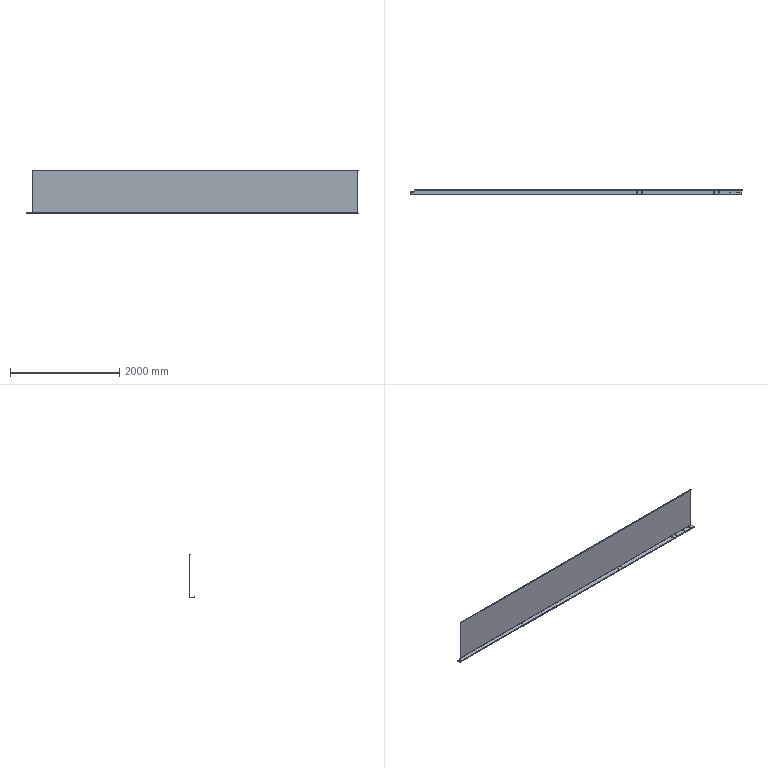Part | STEP file | Microwave Drying Flat Conveyor-CN2500x400-103-101b | 1 solid | 103 faces | box 6084 x 100 x 803 mm | volume 16658166 mm3 | cylinder 77 | plane 25 | spline 1 | commonest cylinder face diameters 6 x27 9 x16 11 x16 7 x10 12 x3 20 x2